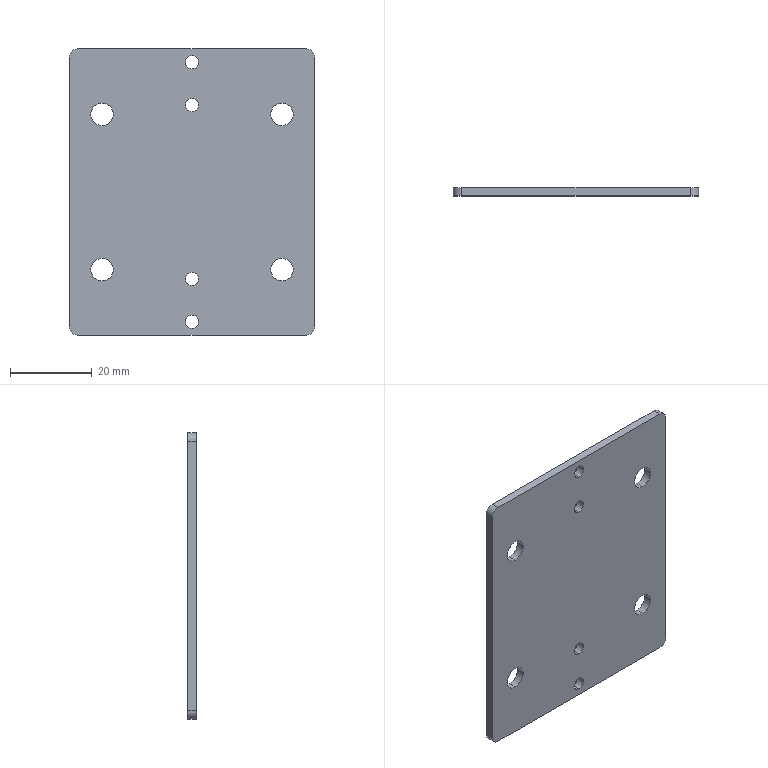Part | SolidWorks | features BaseBody 1 | 1 solid | 26 faces | box 60 x 2 x 70 mm | volume 8139 mm3 | cylinder 20 | plane 6 | commonest cylinder face diameters 3.2 x8 5.5 x8 4 x4
STEP:
#1=CARTESIAN_POINT('',(22.,1.,-16.25));
#2=VERTEX_POINT('',#1);
#3=CARTESIAN_POINT('',(22.,1.,-21.75));
#4=VERTEX_POINT('',#3);
#5=CARTESIAN_POINT('',(22.,1.,-19.));
#6=DIRECTION('',(0.,-1.,0.));
#7=DIRECTION('',(0.,0.,-1.));
#8=AXIS2_PLACEMENT_3D('',#5,#6,#7);
#9=CIRCLE('',#8,2.75);
#10=EDGE_CURVE('',#2,#4,#9,.T.);
#11=ORIENTED_EDGE('',*,*,#10,.F.);
#12=CARTESIAN_POINT('',(22.,-1.,-16.25));
#13=VERTEX_POINT('',#12);
#14=CARTESIAN_POINT('',(22.,1.,-16.25));
#15=DIRECTION('',(0.,-1.,0.));
#16=VECTOR('',#15,1000.);
#17=LINE('',#14,#16);
#18=EDGE_CURVE('',#2,#13,#17,.T.);
#19=ORIENTED_EDGE('',*,*,#18,.T.);
#20=CARTESIAN_POINT('',(22.,-1.,-21.75));
#21=VERTEX_POINT('',#20);
#22=CARTESIAN_POINT('',(22.,-1.,-19.));
#23=DIRECTION('',(0.,1.,0.));
#24=DIRECTION('',(0.,0.,-1.));
#25=AXIS2_PLACEMENT_3D('',#22,#23,#24);
#26=CIRCLE('',#25,2.75);
#27=EDGE_CURVE('',#21,#13,#26,.T.);
#28=ORIENTED_EDGE('',*,*,#27,.F.);
#29=CARTESIAN_POINT('',(22.,1.,-21.75));
#30=DIRECTION('',(0.,-1.,0.));
#31=VECTOR('',#30,1000.);
#32=LINE('',#29,#31);
#33=EDGE_CURVE('',#4,#21,#32,.T.);
#34=ORIENTED_EDGE('',*,*,#33,.F.);
#35=EDGE_LOOP('',(#11,#19,#28,#34));
#36=FACE_OUTER_BOUND('',#35,.T.);
#37=CARTESIAN_POINT('',(22.,1.,-19.));
#38=DIRECTION('',(0.,-1.,0.));
#39=DIRECTION('',(0.,0.,-1.));
#40=AXIS2_PLACEMENT_3D('',#37,#38,#39);
#41=CYLINDRICAL_SURFACE('',#40,2.75);
#42=ADVANCED_FACE('',(#36),#41,.F.);
#43=CARTESIAN_POINT('',(0.,1.,33.35));
#44=VERTEX_POINT('',#43);
#45=CARTESIAN_POINT('',(0.,1.,30.15));
#46=VERTEX_POINT('',#45);
#47=CARTESIAN_POINT('',(0.,1.,31.75));
#48=DIRECTION('',(0.,-1.,0.));
#49=DIRECTION('',(0.,0.,-1.));
#50=AXIS2_PLACEMENT_3D('',#47,#48,#49);
#51=CIRCLE('',#50,1.6);
#52=EDGE_CURVE('',#44,#46,#51,.T.);
#53=ORIENTED_EDGE('',*,*,#52,.F.);
#54=CARTESIAN_POINT('',(0.,-1.,33.35));
#55=VERTEX_POINT('',#54);
#56=CARTESIAN_POINT('',(0.,1.,33.35));
#57=DIRECTION('',(0.,-1.,0.));
#58=VECTOR('',#57,1000.);
#59=LINE('',#56,#58);
#60=EDGE_CURVE('',#44,#55,#59,.T.);
#61=ORIENTED_EDGE('',*,*,#60,.T.);
#62=CARTESIAN_POINT('',(0.,-1.,30.15));
#63=VERTEX_POINT('',#62);
#64=CARTESIAN_POINT('',(0.,-1.,31.75));
#65=DIRECTION('',(0.,1.,0.));
#66=DIRECTION('',(0.,0.,-1.));
#67=AXIS2_PLACEMENT_3D('',#64,#65,#66);
#68=CIRCLE('',#67,1.6);
#69=EDGE_CURVE('',#63,#55,#68,.T.);
#70=ORIENTED_EDGE('',*,*,#69,.F.);
#71=CARTESIAN_POINT('',(0.,1.,30.15));
#72=DIRECTION('',(0.,-1.,0.));
#73=VECTOR('',#72,1000.);
#74=LINE('',#71,#73);
#75=EDGE_CURVE('',#46,#63,#74,.T.);
#76=ORIENTED_EDGE('',*,*,#75,.F.);
#77=EDGE_LOOP('',(#53,#61,#70,#76));
#78=FACE_OUTER_BOUND('',#77,.T.);
#79=CARTESIAN_POINT('',(0.,1.,31.75));
#80=DIRECTION('',(0.,-1.,0.));
#81=DIRECTION('',(0.,0.,-1.));
#82=AXIS2_PLACEMENT_3D('',#79,#80,#81);
#83=CYLINDRICAL_SURFACE('',#82,1.6);
#84=ADVANCED_FACE('',(#78),#83,.F.);
#85=CARTESIAN_POINT('',(0.,1.,-19.65));
#86=VERTEX_POINT('',#85);
#87=CARTESIAN_POINT('',(0.,1.,-22.85));
#88=VERTEX_POINT('',#87);
#89=CARTESIAN_POINT('',(0.,1.,-21.25));
#90=DIRECTION('',(0.,-1.,0.));
#91=DIRECTION('',(0.,0.,-1.));
#92=AXIS2_PLACEMENT_3D('',#89,#90,#91);
#93=CIRCLE('',#92,1.6);
#94=EDGE_CURVE('',#86,#88,#93,.T.);
#95=ORIENTED_EDGE('',*,*,#94,.F.);
#96=CARTESIAN_POINT('',(0.,-1.,-19.65));
#97=VERTEX_POINT('',#96);
#98=CARTESIAN_POINT('',(0.,1.,-19.65));
#99=DIRECTION('',(0.,-1.,0.));
#100=VECTOR('',#99,1000.);
#101=LINE('',#98,#100);
#102=EDGE_CURVE('',#86,#97,#101,.T.);
#103=ORIENTED_EDGE('',*,*,#102,.T.);
#104=CARTESIAN_POINT('',(0.,-1.,-22.85));
#105=VERTEX_POINT('',#104);
#106=CARTESIAN_POINT('',(0.,-1.,-21.25));
#107=DIRECTION('',(0.,1.,0.));
#108=DIRECTION('',(0.,0.,-1.));
#109=AXIS2_PLACEMENT_3D('',#106,#107,#108);
#110=CIRCLE('',#109,1.6);
#111=EDGE_CURVE('',#105,#97,#110,.T.);
#112=ORIENTED_EDGE('',*,*,#111,.F.);
#113=CARTESIAN_POINT('',(0.,1.,-22.85));
#114=DIRECTION('',(0.,-1.,0.));
#115=VECTOR('',#114,1000.);
#116=LINE('',#113,#115);
#117=EDGE_CURVE('',#88,#105,#116,.T.);
#118=ORIENTED_EDGE('',*,*,#117,.F.);
#119=EDGE_LOOP('',(#95,#103,#112,#118));
#120=FACE_OUTER_BOUND('',#119,.T.);
#121=CARTESIAN_POINT('',(0.,1.,-21.25));
#122=DIRECTION('',(0.,-1.,0.));
#123=DIRECTION('',(0.,0.,-1.));
#124=AXIS2_PLACEMENT_3D('',#121,#122,#123);
#125=CYLINDRICAL_SURFACE('',#124,1.6);
#126=ADVANCED_FACE('',(#120),#125,.F.);
#127=CARTESIAN_POINT('',(-22.,1.,21.75));
#128=VERTEX_POINT('',#127);
#129=CARTESIAN_POINT('',(-22.,1.,16.25));
#130=VERTEX_POINT('',#129);
#131=CARTESIAN_POINT('',(-22.,1.,19.));
#132=DIRECTION('',(0.,-1.,0.));
#133=DIRECTION('',(0.,0.,-1.));
#134=AXIS2_PLACEMENT_3D('',#131,#132,#133);
#135=CIRCLE('',#134,2.75);
#136=EDGE_CURVE('',#128,#130,#135,.T.);
#137=ORIENTED_EDGE('',*,*,#136,.F.);
#138=CARTESIAN_POINT('',(-22.,-1.,21.75));
#139=VERTEX_POINT('',#138);
#140=CARTESIAN_POINT('',(-22.,1.,21.75));
#141=DIRECTION('',(0.,-1.,0.));
#142=VECTOR('',#141,1000.);
#143=LINE('',#140,#142);
#144=EDGE_CURVE('',#128,#139,#143,.T.);
#145=ORIENTED_EDGE('',*,*,#144,.T.);
#146=CARTESIAN_POINT('',(-22.,-1.,16.25));
#147=VERTEX_POINT('',#146);
#148=CARTESIAN_POINT('',(-22.,-1.,19.));
#149=DIRECTION('',(0.,1.,0.));
#150=DIRECTION('',(0.,0.,-1.));
#151=AXIS2_PLACEMENT_3D('',#148,#149,#150);
#152=CIRCLE('',#151,2.75);
#153=EDGE_CURVE('',#147,#139,#152,.T.);
#154=ORIENTED_EDGE('',*,*,#153,.F.);
#155=CARTESIAN_POINT('',(-22.,1.,16.25));
#156=DIRECTION('',(0.,-1.,0.));
#157=VECTOR('',#156,1000.);
#158=LINE('',#155,#157);
#159=EDGE_CURVE('',#130,#147,#158,.T.);
#160=ORIENTED_EDGE('',*,*,#159,.F.);
#161=EDGE_LOOP('',(#137,#145,#154,#160));
#162=FACE_OUTER_BOUND('',#161,.T.);
#163=CARTESIAN_POINT('',(-22.,1.,19.));
#164=DIRECTION('',(0.,-1.,0.));
#165=DIRECTION('',(0.,0.,-1.));
#166=AXIS2_PLACEMENT_3D('',#163,#164,#165);
#167=CYLINDRICAL_SURFACE('',#166,2.75);
#168=ADVANCED_FACE('',(#162),#167,.F.);
#169=CARTESIAN_POINT('',(-22.,1.,-16.25));
#170=VERTEX_POINT('',#169);
#171=CARTESIAN_POINT('',(-22.,1.,-21.75));
#172=VERTEX_POINT('',#171);
#173=CARTESIAN_POINT('',(-22.,1.,-19.));
#174=DIRECTION('',(0.,-1.,0.));
#175=DIRECTION('',(0.,0.,-1.));
#176=AXIS2_PLACEMENT_3D('',#173,#174,#175);
#177=CIRCLE('',#176,2.75);
#178=EDGE_CURVE('',#170,#172,#177,.T.);
#179=ORIENTED_EDGE('',*,*,#178,.F.);
#180=CARTESIAN_POINT('',(-22.,-1.,-16.25));
#181=VERTEX_POINT('',#180);
#182=CARTESIAN_POINT('',(-22.,1.,-16.25));
#183=DIRECTION('',(0.,-1.,0.));
#184=VECTOR('',#183,1000.);
#185=LINE('',#182,#184);
#186=EDGE_CURVE('',#170,#181,#185,.T.);
#187=ORIENTED_EDGE('',*,*,#186,.T.);
#188=CARTESIAN_POINT('',(-22.,-1.,-21.75));
#189=VERTEX_POINT('',#188);
#190=CARTESIAN_POINT('',(-22.,-1.,-19.));
#191=DIRECTION('',(0.,1.,0.));
#192=DIRECTION('',(0.,0.,-1.));
#193=AXIS2_PLACEMENT_3D('',#190,#191,#192);
#194=CIRCLE('',#193,2.75);
#195=EDGE_CURVE('',#189,#181,#194,.T.);
#196=ORIENTED_EDGE('',*,*,#195,.F.);
#197=CARTESIAN_POINT('',(-22.,1.,-21.75));
#198=DIRECTION('',(0.,-1.,0.));
#199=VECTOR('',#198,1000.);
#200=LINE('',#197,#199);
#201=EDGE_CURVE('',#172,#189,#200,.T.);
#202=ORIENTED_EDGE('',*,*,#201,.F.);
#203=EDGE_LOOP('',(#179,#187,#196,#202));
#204=FACE_OUTER_BOUND('',#203,.T.);
#205=CARTESIAN_POINT('',(-22.,1.,-19.));
#206=DIRECTION('',(0.,-1.,0.));
#207=DIRECTION('',(0.,0.,-1.));
#208=AXIS2_PLACEMENT_3D('',#205,#206,#207);
#209=CYLINDRICAL_SURFACE('',#208,2.75);
#210=ADVANCED_FACE('',(#204),#209,.F.);
#211=CARTESIAN_POINT('',(0.,1.,-30.15));
#212=VERTEX_POINT('',#211);
#213=CARTESIAN_POINT('',(0.,1.,-33.35));
#214=VERTEX_POINT('',#213);
#215=CARTESIAN_POINT('',(0.,1.,-31.75));
#216=DIRECTION('',(0.,-1.,0.));
#217=DIRECTION('',(0.,0.,-1.));
#218=AXIS2_PLACEMENT_3D('',#215,#216,#217);
#219=CIRCLE('',#218,1.6);
#220=EDGE_CURVE('',#212,#214,#219,.T.);
#221=ORIENTED_EDGE('',*,*,#220,.F.);
#222=CARTESIAN_POINT('',(0.,-1.,-30.15));
#223=VERTEX_POINT('',#222);
#224=CARTESIAN_POINT('',(0.,1.,-30.15));
#225=DIRECTION('',(0.,-1.,0.));
#226=VECTOR('',#225,1000.);
#227=LINE('',#224,#226);
#228=EDGE_CURVE('',#212,#223,#227,.T.);
#229=ORIENTED_EDGE('',*,*,#228,.T.);
#230=CARTESIAN_POINT('',(0.,-1.,-33.35));
#231=VERTEX_POINT('',#230);
#232=CARTESIAN_POINT('',(0.,-1.,-31.75));
#233=DIRECTION('',(0.,1.,0.));
#234=DIRECTION('',(0.,0.,-1.));
#235=AXIS2_PLACEMENT_3D('',#232,#233,#234);
#236=CIRCLE('',#235,1.6);
#237=EDGE_CURVE('',#231,#223,#236,.T.);
#238=ORIENTED_EDGE('',*,*,#237,.F.);
#239=CARTESIAN_POINT('',(0.,1.,-33.35));
#240=DIRECTION('',(0.,-1.,0.));
#241=VECTOR('',#240,1000.);
#242=LINE('',#239,#241);
#243=EDGE_CURVE('',#214,#231,#242,.T.);
#244=ORIENTED_EDGE('',*,*,#243,.F.);
#245=EDGE_LOOP('',(#221,#229,#238,#244));
#246=FACE_OUTER_BOUND('',#245,.T.);
#247=CARTESIAN_POINT('',(0.,1.,-31.75));
#248=DIRECTION('',(0.,-1.,0.));
#249=DIRECTION('',(0.,0.,-1.));
#250=AXIS2_PLACEMENT_3D('',#247,#248,#249);
#251=CYLINDRICAL_SURFACE('',#250,1.6);
#252=ADVANCED_FACE('',(#246),#251,.F.);
#253=CARTESIAN_POINT('',(0.,1.,22.85));
#254=VERTEX_POINT('',#253);
#255=CARTESIAN_POINT('',(0.,1.,19.65));
#256=VERTEX_POINT('',#255);
#257=CARTESIAN_POINT('',(0.,1.,21.25));
#258=DIRECTION('',(0.,-1.,0.));
#259=DIRECTION('',(0.,0.,-1.));
#260=AXIS2_PLACEMENT_3D('',#257,#258,#259);
#261=CIRCLE('',#260,1.6);
#262=EDGE_CURVE('',#254,#256,#261,.T.);
#263=ORIENTED_EDGE('',*,*,#262,.F.);
#264=CARTESIAN_POINT('',(0.,-1.,22.85));
#265=VERTEX_POINT('',#264);
#266=CARTESIAN_POINT('',(0.,1.,22.85));
#267=DIRECTION('',(0.,-1.,0.));
#268=VECTOR('',#267,1000.);
#269=LINE('',#266,#268);
#270=EDGE_CURVE('',#254,#265,#269,.T.);
#271=ORIENTED_EDGE('',*,*,#270,.T.);
#272=CARTESIAN_POINT('',(0.,-1.,19.65));
#273=VERTEX_POINT('',#272);
#274=CARTESIAN_POINT('',(0.,-1.,21.25));
#275=DIRECTION('',(0.,1.,0.));
#276=DIRECTION('',(0.,0.,-1.));
#277=AXIS2_PLACEMENT_3D('',#274,#275,#276);
#278=CIRCLE('',#277,1.6);
#279=EDGE_CURVE('',#273,#265,#278,.T.);
#280=ORIENTED_EDGE('',*,*,#279,.F.);
#281=CARTESIAN_POINT('',(0.,1.,19.65));
#282=DIRECTION('',(0.,-1.,0.));
#283=VECTOR('',#282,1000.);
#284=LINE('',#281,#283);
#285=EDGE_CURVE('',#256,#273,#284,.T.);
#286=ORIENTED_EDGE('',*,*,#285,.F.);
#287=EDGE_LOOP('',(#263,#271,#280,#286));
#288=FACE_OUTER_BOUND('',#287,.T.);
#289=CARTESIAN_POINT('',(0.,1.,21.25));
#290=DIRECTION('',(0.,-1.,0.));
#291=DIRECTION('',(0.,0.,-1.));
#292=AXIS2_PLACEMENT_3D('',#289,#290,#291);
#293=CYLINDRICAL_SURFACE('',#292,1.6);
#294=ADVANCED_FACE('',(#288),#293,.F.);
#295=CARTESIAN_POINT('',(22.,1.,21.75));
#296=VERTEX_POINT('',#295);
#297=CARTESIAN_POINT('',(22.,1.,16.25));
#298=VERTEX_POINT('',#297);
#299=CARTESIAN_POINT('',(22.,1.,19.));
#300=DIRECTION('',(0.,-1.,0.));
#301=DIRECTION('',(0.,0.,-1.));
#302=AXIS2_PLACEMENT_3D('',#299,#300,#301);
#303=CIRCLE('',#302,2.75);
#304=EDGE_CURVE('',#296,#298,#303,.T.);
#305=ORIENTED_EDGE('',*,*,#304,.F.);
#306=CARTESIAN_POINT('',(22.,-1.,21.75));
#307=VERTEX_POINT('',#306);
#308=CARTESIAN_POINT('',(22.,1.,21.75));
#309=DIRECTION('',(0.,-1.,0.));
#310=VECTOR('',#309,1000.);
#311=LINE('',#308,#310);
#312=EDGE_CURVE('',#296,#307,#311,.T.);
#313=ORIENTED_EDGE('',*,*,#312,.T.);
#314=CARTESIAN_POINT('',(22.,-1.,16.25));
#315=VERTEX_POINT('',#314);
#316=CARTESIAN_POINT('',(22.,-1.,19.));
#317=DIRECTION('',(0.,1.,0.));
#318=DIRECTION('',(0.,0.,-1.));
#319=AXIS2_PLACEMENT_3D('',#316,#317,#318);
#320=CIRCLE('',#319,2.75);
#321=EDGE_CURVE('',#315,#307,#320,.T.);
#322=ORIENTED_EDGE('',*,*,#321,.F.);
#323=CARTESIAN_POINT('',(22.,1.,16.25));
#324=DIRECTION('',(0.,-1.,0.));
#325=VECTOR('',#324,1000.);
#326=LINE('',#323,#325);
#327=EDGE_CURVE('',#298,#315,#326,.T.);
#328=ORIENTED_EDGE('',*,*,#327,.F.);
#329=EDGE_LOOP('',(#305,#313,#322,#328));
#330=FACE_OUTER_BOUND('',#329,.T.);
#331=CARTESIAN_POINT('',(22.,1.,19.));
#332=DIRECTION('',(0.,-1.,0.));
#333=DIRECTION('',(0.,0.,-1.));
#334=AXIS2_PLACEMENT_3D('',#331,#332,#333);
#335=CYLINDRICAL_SURFACE('',#334,2.75);
#336=ADVANCED_FACE('',(#330),#335,.F.);
#337=CARTESIAN_POINT('',(22.,1.,-19.));
#338=DIRECTION('',(0.,-1.,0.));
#339=DIRECTION('',(0.,0.,-1.));
#340=AXIS2_PLACEMENT_3D('',#337,#338,#339);
#341=CIRCLE('',#340,2.75);
#342=EDGE_CURVE('',#4,#2,#341,.T.);
#343=ORIENTED_EDGE('',*,*,#342,.T.);
#344=ORIENTED_EDGE('',*,*,#10,.T.);
#345=EDGE_LOOP('',(#343,#344));
#346=FACE_BOUND('',#345,.T.);
#347=CARTESIAN_POINT('',(0.,1.,31.75));
#348=DIRECTION('',(0.,-1.,0.));
#349=DIRECTION('',(0.,0.,-1.));
#350=AXIS2_PLACEMENT_3D('',#347,#348,#349);
#351=CIRCLE('',#350,1.6);
#352=EDGE_CURVE('',#46,#44,#351,.T.);
#353=ORIENTED_EDGE('',*,*,#352,.T.);
#354=ORIENTED_EDGE('',*,*,#52,.T.);
#355=EDGE_LOOP('',(#353,#354));
#356=FACE_BOUND('',#355,.T.);
#357=CARTESIAN_POINT('',(0.,1.,-21.25));
#358=DIRECTION('',(0.,-1.,0.));
#359=DIRECTION('',(0.,0.,-1.));
#360=AXIS2_PLACEMENT_3D('',#357,#358,#359);
#361=CIRCLE('',#360,1.6);
#362=EDGE_CURVE('',#88,#86,#361,.T.);
#363=ORIENTED_EDGE('',*,*,#362,.T.);
#364=ORIENTED_EDGE('',*,*,#94,.T.);
#365=EDGE_LOOP('',(#363,#364));
#366=FACE_BOUND('',#365,.T.);
#367=CARTESIAN_POINT('',(-22.,1.,19.));
#368=DIRECTION('',(0.,-1.,0.));
#369=DIRECTION('',(0.,0.,-1.));
#370=AXIS2_PLACEMENT_3D('',#367,#368,#369);
#371=CIRCLE('',#370,2.75);
#372=EDGE_CURVE('',#130,#128,#371,.T.);
#373=ORIENTED_EDGE('',*,*,#372,.T.);
#374=ORIENTED_EDGE('',*,*,#136,.T.);
#375=EDGE_LOOP('',(#373,#374));
#376=FACE_BOUND('',#375,.T.);
#377=CARTESIAN_POINT('',(-30.,1.,-33.));
#378=VERTEX_POINT('',#377);
#379=CARTESIAN_POINT('',(-30.,1.,33.));
#380=VERTEX_POINT('',#379);
#381=CARTESIAN_POINT('',(-30.,1.,0.));
#382=DIRECTION('',(0.,0.,1.));
#383=VECTOR('',#382,1000.);
#384=LINE('',#381,#383);
#385=EDGE_CURVE('',#378,#380,#384,.T.);
#386=ORIENTED_EDGE('',*,*,#385,.T.);
#387=CARTESIAN_POINT('',(-28.,1.,35.));
#388=VERTEX_POINT('',#387);
#389=CARTESIAN_POINT('',(-28.,1.,33.));
#390=DIRECTION('',(0.,1.,0.));
#391=DIRECTION('',(0.,0.,-1.));
#392=AXIS2_PLACEMENT_3D('',#389,#390,#391);
#393=CIRCLE('',#392,2.);
#394=EDGE_CURVE('',#380,#388,#393,.T.);
#395=ORIENTED_EDGE('',*,*,#394,.T.);
#396=CARTESIAN_POINT('',(28.,1.,35.));
#397=VERTEX_POINT('',#396);
#398=CARTESIAN_POINT('',(0.,1.,35.));
#399=DIRECTION('',(1.,0.,0.));
#400=VECTOR('',#399,1000.);
#401=LINE('',#398,#400);
#402=EDGE_CURVE('',#388,#397,#401,.T.);
#403=ORIENTED_EDGE('',*,*,#402,.T.);
#404=CARTESIAN_POINT('',(30.,1.,33.));
#405=VERTEX_POINT('',#404);
#406=CARTESIAN_POINT('',(28.,1.,33.));
#407=DIRECTION('',(0.,1.,0.));
#408=DIRECTION('',(0.,0.,-1.));
#409=AXIS2_PLACEMENT_3D('',#406,#407,#408);
#410=CIRCLE('',#409,2.);
#411=EDGE_CURVE('',#397,#405,#410,.T.);
#412=ORIENTED_EDGE('',*,*,#411,.T.);
#413=CARTESIAN_POINT('',(30.,1.,-33.));
#414=VERTEX_POINT('',#413);
#415=CARTESIAN_POINT('',(30.,1.,0.));
#416=DIRECTION('',(0.,0.,-1.));
#417=VECTOR('',#416,1000.);
#418=LINE('',#415,#417);
#419=EDGE_CURVE('',#405,#414,#418,.T.);
#420=ORIENTED_EDGE('',*,*,#419,.T.);
#421=CARTESIAN_POINT('',(28.,1.,-35.));
#422=VERTEX_POINT('',#421);
#423=CARTESIAN_POINT('',(28.,1.,-33.));
#424=DIRECTION('',(0.,1.,0.));
#425=DIRECTION('',(0.,0.,-1.));
#426=AXIS2_PLACEMENT_3D('',#423,#424,#425);
#427=CIRCLE('',#426,2.);
#428=EDGE_CURVE('',#414,#422,#427,.T.);
#429=ORIENTED_EDGE('',*,*,#428,.T.);
#430=CARTESIAN_POINT('',(-28.,1.,-35.));
#431=VERTEX_POINT('',#430);
#432=CARTESIAN_POINT('',(0.,1.,-35.));
#433=DIRECTION('',(-1.,0.,0.));
#434=VECTOR('',#433,1000.);
#435=LINE('',#432,#434);
#436=EDGE_CURVE('',#422,#431,#435,.T.);
#437=ORIENTED_EDGE('',*,*,#436,.T.);
#438=CARTESIAN_POINT('',(-28.,1.,-33.));
#439=DIRECTION('',(0.,1.,0.));
#440=DIRECTION('',(0.,0.,-1.));
#441=AXIS2_PLACEMENT_3D('',#438,#439,#440);
#442=CIRCLE('',#441,2.);
#443=EDGE_CURVE('',#431,#378,#442,.T.);
#444=ORIENTED_EDGE('',*,*,#443,.T.);
#445=EDGE_LOOP('',(#386,#395,#403,#412,#420,#429,#437,#444));
#446=FACE_OUTER_BOUND('',#445,.T.);
#447=CARTESIAN_POINT('',(-22.,1.,-19.));
#448=DIRECTION('',(0.,-1.,0.));
#449=DIRECTION('',(0.,0.,-1.));
#450=AXIS2_PLACEMENT_3D('',#447,#448,#449);
#451=CIRCLE('',#450,2.75);
#452=EDGE_CURVE('',#172,#170,#451,.T.);
#453=ORIENTED_EDGE('',*,*,#452,.T.);
#454=ORIENTED_EDGE('',*,*,#178,.T.);
#455=EDGE_LOOP('',(#453,#454));
#456=FACE_BOUND('',#455,.T.);
#457=CARTESIAN_POINT('',(0.,1.,-31.75));
#458=DIRECTION('',(0.,-1.,0.));
#459=DIRECTION('',(0.,0.,-1.));
#460=AXIS2_PLACEMENT_3D('',#457,#458,#459);
#461=CIRCLE('',#460,1.6);
#462=EDGE_CURVE('',#214,#212,#461,.T.);
#463=ORIENTED_EDGE('',*,*,#462,.T.);
#464=ORIENTED_EDGE('',*,*,#220,.T.);
#465=EDGE_LOOP('',(#463,#464));
#466=FACE_BOUND('',#465,.T.);
#467=CARTESIAN_POINT('',(0.,1.,21.25));
#468=DIRECTION('',(0.,-1.,0.));
#469=DIRECTION('',(0.,0.,-1.));
#470=AXIS2_PLACEMENT_3D('',#467,#468,#469);
#471=CIRCLE('',#470,1.6);
#472=EDGE_CURVE('',#256,#254,#471,.T.);
#473=ORIENTED_EDGE('',*,*,#472,.T.);
#474=ORIENTED_EDGE('',*,*,#262,.T.);
#475=EDGE_LOOP('',(#473,#474));
#476=FACE_BOUND('',#475,.T.);
#477=CARTESIAN_POINT('',(22.,1.,19.));
#478=DIRECTION('',(0.,-1.,0.));
#479=DIRECTION('',(0.,0.,-1.));
#480=AXIS2_PLACEMENT_3D('',#477,#478,#479);
#481=CIRCLE('',#480,2.75);
#482=EDGE_CURVE('',#298,#296,#481,.T.);
#483=ORIENTED_EDGE('',*,*,#482,.T.);
#484=ORIENTED_EDGE('',*,*,#304,.T.);
#485=EDGE_LOOP('',(#483,#484));
#486=FACE_BOUND('',#485,.T.);
#487=CARTESIAN_POINT('',(0.,1.,0.));
#488=DIRECTION('',(0.,1.,0.));
#489=DIRECTION('',(0.,0.,1.));
#490=AXIS2_PLACEMENT_3D('',#487,#488,#489);
#491=PLANE('',#490);
#492=ADVANCED_FACE('',(#346,#356,#366,#376,#446,#456,#466,#476,#486),#491,.T.);
#493=ORIENTED_EDGE('',*,*,#18,.F.);
#494=ORIENTED_EDGE('',*,*,#342,.F.);
#495=ORIENTED_EDGE('',*,*,#33,.T.);
#496=CARTESIAN_POINT('',(22.,-1.,-19.));
#497=DIRECTION('',(0.,1.,0.));
#498=DIRECTION('',(0.,0.,-1.));
#499=AXIS2_PLACEMENT_3D('',#496,#497,#498);
#500=CIRCLE('',#499,2.75);
#501=EDGE_CURVE('',#13,#21,#500,.T.);
#502=ORIENTED_EDGE('',*,*,#501,.F.);
#503=EDGE_LOOP('',(#493,#494,#495,#502));
#504=FACE_OUTER_BOUND('',#503,.T.);
#505=CARTESIAN_POINT('',(22.,1.,-19.));
#506=DIRECTION('',(0.,-1.,0.));
#507=DIRECTION('',(0.,0.,-1.));
#508=AXIS2_PLACEMENT_3D('',#505,#506,#507);
#509=CYLINDRICAL_SURFACE('',#508,2.75);
#510=ADVANCED_FACE('',(#504),#509,.F.);
#511=ORIENTED_EDGE('',*,*,#60,.F.);
#512=ORIENTED_EDGE('',*,*,#352,.F.);
#513=ORIENTED_EDGE('',*,*,#75,.T.);
#514=CARTESIAN_POINT('',(0.,-1.,31.75));
#515=DIRECTION('',(0.,1.,0.));
#516=DIRECTION('',(0.,0.,-1.));
#517=AXIS2_PLACEMENT_3D('',#514,#515,#516);
#518=CIRCLE('',#517,1.6);
#519=EDGE_CURVE('',#55,#63,#518,.T.);
#520=ORIENTED_EDGE('',*,*,#519,.F.);
#521=EDGE_LOOP('',(#511,#512,#513,#520));
#522=FACE_OUTER_BOUND('',#521,.T.);
#523=CARTESIAN_POINT('',(0.,1.,31.75));
#524=DIRECTION('',(0.,-1.,0.));
#525=DIRECTION('',(0.,0.,-1.));
#526=AXIS2_PLACEMENT_3D('',#523,#524,#525);
#527=CYLINDRICAL_SURFACE('',#526,1.6);
#528=ADVANCED_FACE('',(#522),#527,.F.);
#529=ORIENTED_EDGE('',*,*,#102,.F.);
#530=ORIENTED_EDGE('',*,*,#362,.F.);
#531=ORIENTED_EDGE('',*,*,#117,.T.);
#532=CARTESIAN_POINT('',(0.,-1.,-21.25));
#533=DIRECTION('',(0.,1.,0.));
#534=DIRECTION('',(0.,0.,-1.));
#535=AXIS2_PLACEMENT_3D('',#532,#533,#534);
#536=CIRCLE('',#535,1.6);
#537=EDGE_CURVE('',#97,#105,#536,.T.);
#538=ORIENTED_EDGE('',*,*,#537,.F.);
#539=EDGE_LOOP('',(#529,#530,#531,#538));
#540=FACE_OUTER_BOUND('',#539,.T.);
#541=CARTESIAN_POINT('',(0.,1.,-21.25));
#542=DIRECTION('',(0.,-1.,0.));
#543=DIRECTION('',(0.,0.,-1.));
#544=AXIS2_PLACEMENT_3D('',#541,#542,#543);
#545=CYLINDRICAL_SURFACE('',#544,1.6);
#546=ADVANCED_FACE('',(#540),#545,.F.);
#547=ORIENTED_EDGE('',*,*,#144,.F.);
#548=ORIENTED_EDGE('',*,*,#372,.F.);
#549=ORIENTED_EDGE('',*,*,#159,.T.);
#550=CARTESIAN_POINT('',(-22.,-1.,19.));
#551=DIRECTION('',(0.,1.,0.));
#552=DIRECTION('',(0.,0.,-1.));
#553=AXIS2_PLACEMENT_3D('',#550,#551,#552);
#554=CIRCLE('',#553,2.75);
#555=EDGE_CURVE('',#139,#147,#554,.T.);
#556=ORIENTED_EDGE('',*,*,#555,.F.);
#557=EDGE_LOOP('',(#547,#548,#549,#556));
#558=FACE_OUTER_BOUND('',#557,.T.);
#559=CARTESIAN_POINT('',(-22.,1.,19.));
#560=DIRECTION('',(0.,-1.,0.));
#561=DIRECTION('',(0.,0.,-1.));
#562=AXIS2_PLACEMENT_3D('',#559,#560,#561);
#563=CYLINDRICAL_SURFACE('',#562,2.75);
#564=ADVANCED_FACE('',(#558),#563,.F.);
#565=CARTESIAN_POINT('',(-30.,-1.,33.));
#566=VERTEX_POINT('',#565);
#567=CARTESIAN_POINT('',(-28.,-1.,35.));
#568=VERTEX_POINT('',#567);
#569=CARTESIAN_POINT('',(-28.,-1.,33.));
#570=DIRECTION('',(0.,1.,0.));
#571=DIRECTION('',(0.,0.,-1.));
#572=AXIS2_PLACEMENT_3D('',#569,#570,#571);
#573=CIRCLE('',#572,2.);
#574=EDGE_CURVE('',#566,#568,#573,.T.);
#575=ORIENTED_EDGE('',*,*,#574,.T.);
#576=CARTESIAN_POINT('',(-28.,1.,35.));
#577=DIRECTION('',(0.,1.,0.));
#578=VECTOR('',#577,1000.);
#579=LINE('',#576,#578);
#580=EDGE_CURVE('',#568,#388,#579,.T.);
#581=ORIENTED_EDGE('',*,*,#580,.T.);
#582=ORIENTED_EDGE('',*,*,#394,.F.);
#583=CARTESIAN_POINT('',(-30.,1.,33.));
#584=DIRECTION('',(0.,-1.,0.));
#585=VECTOR('',#584,1000.);
#586=LINE('',#583,#585);
#587=EDGE_CURVE('',#380,#566,#586,.T.);
#588=ORIENTED_EDGE('',*,*,#587,.T.);
#589=EDGE_LOOP('',(#575,#581,#582,#588));
#590=FACE_OUTER_BOUND('',#589,.T.);
#591=CARTESIAN_POINT('',(-28.,1.,33.));
#592=DIRECTION('',(0.,-1.,0.));
#593=DIRECTION('',(0.,0.,-1.));
#594=AXIS2_PLACEMENT_3D('',#591,#592,#593);
#595=CYLINDRICAL_SURFACE('',#594,2.);
#596=ADVANCED_FACE('',(#590),#595,.T.);
#597=ORIENTED_EDGE('',*,*,#587,.F.);
#598=ORIENTED_EDGE('',*,*,#385,.F.);
#599=CARTESIAN_POINT('',(-30.,-1.,-33.));
#600=VERTEX_POINT('',#599);
#601=CARTESIAN_POINT('',(-30.,1.,-33.));
#602=DIRECTION('',(0.,1.,0.));
#603=VECTOR('',#602,1000.);
#604=LINE('',#601,#603);
#605=EDGE_CURVE('',#600,#378,#604,.T.);
#606=ORIENTED_EDGE('',*,*,#605,.F.);
#607=CARTESIAN_POINT('',(-30.,-1.,35.));
#608=DIRECTION('',(0.,0.,-1.));
#609=VECTOR('',#608,1000.);
#610=LINE('',#607,#609);
#611=EDGE_CURVE('',#566,#600,#610,.T.);
#612=ORIENTED_EDGE('',*,*,#611,.F.);
#613=EDGE_LOOP('',(#597,#598,#606,#612));
#614=FACE_OUTER_BOUND('',#613,.T.);
#615=CARTESIAN_POINT('',(-30.,1.,35.));
#616=DIRECTION('',(1.,0.,0.));
#617=DIRECTION('',(0.,0.,-1.));
#618=AXIS2_PLACEMENT_3D('',#615,#616,#617);
#619=PLANE('',#618);
#620=ADVANCED_FACE('',(#614),#619,.F.);
#621=CARTESIAN_POINT('',(-28.,-1.,-35.));
#622=VERTEX_POINT('',#621);
#623=CARTESIAN_POINT('',(-28.,-1.,-33.));
#624=DIRECTION('',(0.,1.,0.));
#625=DIRECTION('',(0.,0.,-1.));
#626=AXIS2_PLACEMENT_3D('',#623,#624,#625);
#627=CIRCLE('',#626,2.);
#628=EDGE_CURVE('',#622,#600,#627,.T.);
#629=ORIENTED_EDGE('',*,*,#628,.T.);
#630=ORIENTED_EDGE('',*,*,#605,.T.);
#631=ORIENTED_EDGE('',*,*,#443,.F.);
#632=CARTESIAN_POINT('',(-28.,1.,-35.));
#633=DIRECTION('',(0.,-1.,0.));
#634=VECTOR('',#633,1000.);
#635=LINE('',#632,#634);
#636=EDGE_CURVE('',#431,#622,#635,.T.);
#637=ORIENTED_EDGE('',*,*,#636,.T.);
#638=EDGE_LOOP('',(#629,#630,#631,#637));
#639=FACE_OUTER_BOUND('',#638,.T.);
#640=CARTESIAN_POINT('',(-28.,1.,-33.));
#641=DIRECTION('',(0.,-1.,0.));
#642=DIRECTION('',(0.,0.,-1.));
#643=AXIS2_PLACEMENT_3D('',#640,#641,#642);
#644=CYLINDRICAL_SURFACE('',#643,2.);
#645=ADVANCED_FACE('',(#639),#644,.T.);
#646=CARTESIAN_POINT('',(28.,-1.,-35.));
#647=VERTEX_POINT('',#646);
#648=CARTESIAN_POINT('',(28.,1.,-35.));
#649=DIRECTION('',(0.,1.,0.));
#650=VECTOR('',#649,1000.);
#651=LINE('',#648,#650);
#652=EDGE_CURVE('',#647,#422,#651,.T.);
#653=ORIENTED_EDGE('',*,*,#652,.F.);
#654=CARTESIAN_POINT('',(30.,-1.,-35.));
#655=DIRECTION('',(1.,0.,0.));
#656=VECTOR('',#655,1000.);
#657=LINE('',#654,#656);
#658=EDGE_CURVE('',#622,#647,#657,.T.);
#659=ORIENTED_EDGE('',*,*,#658,.F.);
#660=ORIENTED_EDGE('',*,*,#636,.F.);
#661=ORIENTED_EDGE('',*,*,#436,.F.);
#662=EDGE_LOOP('',(#653,#659,#660,#661));
#663=FACE_OUTER_BOUND('',#662,.T.);
#664=CARTESIAN_POINT('',(30.,1.,-35.));
#665=DIRECTION('',(0.,0.,1.));
#666=DIRECTION('',(1.,0.,0.));
#667=AXIS2_PLACEMENT_3D('',#664,#665,#666);
#668=PLANE('',#667);
#669=ADVANCED_FACE('',(#663),#668,.F.);
#670=CARTESIAN_POINT('',(30.,-1.,-33.));
#671=VERTEX_POINT('',#670);
#672=CARTESIAN_POINT('',(28.,-1.,-33.));
#673=DIRECTION('',(0.,1.,0.));
#674=DIRECTION('',(0.,0.,-1.));
#675=AXIS2_PLACEMENT_3D('',#672,#673,#674);
#676=CIRCLE('',#675,2.);
#677=EDGE_CURVE('',#671,#647,#676,.T.);
#678=ORIENTED_EDGE('',*,*,#677,.T.);
#679=ORIENTED_EDGE('',*,*,#652,.T.);
#680=ORIENTED_EDGE('',*,*,#428,.F.);
#681=CARTESIAN_POINT('',(30.,1.,-33.));
#682=DIRECTION('',(0.,-1.,0.));
#683=VECTOR('',#682,1000.);
#684=LINE('',#681,#683);
#685=EDGE_CURVE('',#414,#671,#684,.T.);
#686=ORIENTED_EDGE('',*,*,#685,.T.);
#687=EDGE_LOOP('',(#678,#679,#680,#686));
#688=FACE_OUTER_BOUND('',#687,.T.);
#689=CARTESIAN_POINT('',(28.,1.,-33.));
#690=DIRECTION('',(0.,-1.,0.));
#691=DIRECTION('',(0.,0.,-1.));
#692=AXIS2_PLACEMENT_3D('',#689,#690,#691);
#693=CYLINDRICAL_SURFACE('',#692,2.);
#694=ADVANCED_FACE('',(#688),#693,.T.);
#695=CARTESIAN_POINT('',(30.,-1.,33.));
#696=VERTEX_POINT('',#695);
#697=CARTESIAN_POINT('',(30.,1.,33.));
#698=DIRECTION('',(0.,1.,0.));
#699=VECTOR('',#698,1000.);
#700=LINE('',#697,#699);
#701=EDGE_CURVE('',#696,#405,#700,.T.);
#702=ORIENTED_EDGE('',*,*,#701,.F.);
#703=CARTESIAN_POINT('',(30.,-1.,35.));
#704=DIRECTION('',(0.,0.,1.));
#705=VECTOR('',#704,1000.);
#706=LINE('',#703,#705);
#707=EDGE_CURVE('',#671,#696,#706,.T.);
#708=ORIENTED_EDGE('',*,*,#707,.F.);
#709=ORIENTED_EDGE('',*,*,#685,.F.);
#710=ORIENTED_EDGE('',*,*,#419,.F.);
#711=EDGE_LOOP('',(#702,#708,#709,#710));
#712=FACE_OUTER_BOUND('',#711,.T.);
#713=CARTESIAN_POINT('',(30.,1.,35.));
#714=DIRECTION('',(-1.,0.,0.));
#715=DIRECTION('',(0.,0.,1.));
#716=AXIS2_PLACEMENT_3D('',#713,#714,#715);
#717=PLANE('',#716);
#718=ADVANCED_FACE('',(#712),#717,.F.);
#719=CARTESIAN_POINT('',(28.,-1.,35.));
#720=VERTEX_POINT('',#719);
#721=CARTESIAN_POINT('',(28.,-1.,33.));
#722=DIRECTION('',(0.,1.,0.));
#723=DIRECTION('',(0.,0.,-1.));
#724=AXIS2_PLACEMENT_3D('',#721,#722,#723);
#725=CIRCLE('',#724,2.);
#726=EDGE_CURVE('',#720,#696,#725,.T.);
#727=ORIENTED_EDGE('',*,*,#726,.T.);
#728=ORIENTED_EDGE('',*,*,#701,.T.);
#729=ORIENTED_EDGE('',*,*,#411,.F.);
#730=CARTESIAN_POINT('',(28.,1.,35.));
#731=DIRECTION('',(0.,-1.,0.));
#732=VECTOR('',#731,1000.);
#733=LINE('',#730,#732);
#734=EDGE_CURVE('',#397,#720,#733,.T.);
#735=ORIENTED_EDGE('',*,*,#734,.T.);
#736=EDGE_LOOP('',(#727,#728,#729,#735));
#737=FACE_OUTER_BOUND('',#736,.T.);
#738=CARTESIAN_POINT('',(28.,1.,33.));
#739=DIRECTION('',(0.,-1.,0.));
#740=DIRECTION('',(0.,0.,-1.));
#741=AXIS2_PLACEMENT_3D('',#738,#739,#740);
#742=CYLINDRICAL_SURFACE('',#741,2.);
#743=ADVANCED_FACE('',(#737),#742,.T.);
#744=ORIENTED_EDGE('',*,*,#734,.F.);
#745=ORIENTED_EDGE('',*,*,#402,.F.);
#746=ORIENTED_EDGE('',*,*,#580,.F.);
#747=CARTESIAN_POINT('',(30.,-1.,35.));
#748=DIRECTION('',(-1.,0.,0.));
#749=VECTOR('',#748,1000.);
#750=LINE('',#747,#749);
#751=EDGE_CURVE('',#720,#568,#750,.T.);
#752=ORIENTED_EDGE('',*,*,#751,.F.);
#753=EDGE_LOOP('',(#744,#745,#746,#752));
#754=FACE_OUTER_BOUND('',#753,.T.);
#755=CARTESIAN_POINT('',(30.,1.,35.));
#756=DIRECTION('',(0.,0.,-1.));
#757=DIRECTION('',(-1.,0.,0.));
#758=AXIS2_PLACEMENT_3D('',#755,#756,#757);
#759=PLANE('',#758);
#760=ADVANCED_FACE('',(#754),#759,.F.);
#761=ORIENTED_EDGE('',*,*,#186,.F.);
#762=ORIENTED_EDGE('',*,*,#452,.F.);
#763=ORIENTED_EDGE('',*,*,#201,.T.);
#764=CARTESIAN_POINT('',(-22.,-1.,-19.));
#765=DIRECTION('',(0.,1.,0.));
#766=DIRECTION('',(0.,0.,-1.));
#767=AXIS2_PLACEMENT_3D('',#764,#765,#766);
#768=CIRCLE('',#767,2.75);
#769=EDGE_CURVE('',#181,#189,#768,.T.);
#770=ORIENTED_EDGE('',*,*,#769,.F.);
#771=EDGE_LOOP('',(#761,#762,#763,#770));
#772=FACE_OUTER_BOUND('',#771,.T.);
#773=CARTESIAN_POINT('',(-22.,1.,-19.));
#774=DIRECTION('',(0.,-1.,0.));
#775=DIRECTION('',(0.,0.,-1.));
#776=AXIS2_PLACEMENT_3D('',#773,#774,#775);
#777=CYLINDRICAL_SURFACE('',#776,2.75);
#778=ADVANCED_FACE('',(#772),#777,.F.);
#779=ORIENTED_EDGE('',*,*,#228,.F.);
#780=ORIENTED_EDGE('',*,*,#462,.F.);
#781=ORIENTED_EDGE('',*,*,#243,.T.);
#782=CARTESIAN_POINT('',(0.,-1.,-31.75));
#783=DIRECTION('',(0.,1.,0.));
#784=DIRECTION('',(0.,0.,-1.));
#785=AXIS2_PLACEMENT_3D('',#782,#783,#784);
#786=CIRCLE('',#785,1.6);
#787=EDGE_CURVE('',#223,#231,#786,.T.);
#788=ORIENTED_EDGE('',*,*,#787,.F.);
#789=EDGE_LOOP('',(#779,#780,#781,#788));
#790=FACE_OUTER_BOUND('',#789,.T.);
#791=CARTESIAN_POINT('',(0.,1.,-31.75));
#792=DIRECTION('',(0.,-1.,0.));
#793=DIRECTION('',(0.,0.,-1.));
#794=AXIS2_PLACEMENT_3D('',#791,#792,#793);
#795=CYLINDRICAL_SURFACE('',#794,1.6);
#796=ADVANCED_FACE('',(#790),#795,.F.);
#797=ORIENTED_EDGE('',*,*,#270,.F.);
#798=ORIENTED_EDGE('',*,*,#472,.F.);
#799=ORIENTED_EDGE('',*,*,#285,.T.);
#800=CARTESIAN_POINT('',(0.,-1.,21.25));
#801=DIRECTION('',(0.,1.,0.));
#802=DIRECTION('',(0.,0.,-1.));
#803=AXIS2_PLACEMENT_3D('',#800,#801,#802);
#804=CIRCLE('',#803,1.6);
#805=EDGE_CURVE('',#265,#273,#804,.T.);
#806=ORIENTED_EDGE('',*,*,#805,.F.);
#807=EDGE_LOOP('',(#797,#798,#799,#806));
#808=FACE_OUTER_BOUND('',#807,.T.);
#809=CARTESIAN_POINT('',(0.,1.,21.25));
#810=DIRECTION('',(0.,-1.,0.));
#811=DIRECTION('',(0.,0.,-1.));
#812=AXIS2_PLACEMENT_3D('',#809,#810,#811);
#813=CYLINDRICAL_SURFACE('',#812,1.6);
#814=ADVANCED_FACE('',(#808),#813,.F.);
#815=ORIENTED_EDGE('',*,*,#312,.F.);
#816=ORIENTED_EDGE('',*,*,#482,.F.);
#817=ORIENTED_EDGE('',*,*,#327,.T.);
#818=CARTESIAN_POINT('',(22.,-1.,19.));
#819=DIRECTION('',(0.,1.,0.));
#820=DIRECTION('',(0.,0.,-1.));
#821=AXIS2_PLACEMENT_3D('',#818,#819,#820);
#822=CIRCLE('',#821,2.75);
#823=EDGE_CURVE('',#307,#315,#822,.T.);
#824=ORIENTED_EDGE('',*,*,#823,.F.);
#825=EDGE_LOOP('',(#815,#816,#817,#824));
#826=FACE_OUTER_BOUND('',#825,.T.);
#827=CARTESIAN_POINT('',(22.,1.,19.));
#828=DIRECTION('',(0.,-1.,0.));
#829=DIRECTION('',(0.,0.,-1.));
#830=AXIS2_PLACEMENT_3D('',#827,#828,#829);
#831=CYLINDRICAL_SURFACE('',#830,2.75);
#832=ADVANCED_FACE('',(#826),#831,.F.);
#833=ORIENTED_EDGE('',*,*,#27,.T.);
#834=ORIENTED_EDGE('',*,*,#501,.T.);
#835=EDGE_LOOP('',(#833,#834));
#836=FACE_BOUND('',#835,.T.);
#837=ORIENTED_EDGE('',*,*,#321,.T.);
#838=ORIENTED_EDGE('',*,*,#823,.T.);
#839=EDGE_LOOP('',(#837,#838));
#840=FACE_BOUND('',#839,.T.);
#841=ORIENTED_EDGE('',*,*,#69,.T.);
#842=ORIENTED_EDGE('',*,*,#519,.T.);
#843=EDGE_LOOP('',(#841,#842));
#844=FACE_BOUND('',#843,.T.);
#845=ORIENTED_EDGE('',*,*,#279,.T.);
#846=ORIENTED_EDGE('',*,*,#805,.T.);
#847=EDGE_LOOP('',(#845,#846));
#848=FACE_BOUND('',#847,.T.);
#849=ORIENTED_EDGE('',*,*,#111,.T.);
#850=ORIENTED_EDGE('',*,*,#537,.T.);
#851=EDGE_LOOP('',(#849,#850));
#852=FACE_BOUND('',#851,.T.);
#853=ORIENTED_EDGE('',*,*,#237,.T.);
#854=ORIENTED_EDGE('',*,*,#787,.T.);
#855=EDGE_LOOP('',(#853,#854));
#856=FACE_BOUND('',#855,.T.);
#857=ORIENTED_EDGE('',*,*,#153,.T.);
#858=ORIENTED_EDGE('',*,*,#555,.T.);
#859=EDGE_LOOP('',(#857,#858));
#860=FACE_BOUND('',#859,.T.);
#861=ORIENTED_EDGE('',*,*,#195,.T.);
#862=ORIENTED_EDGE('',*,*,#769,.T.);
#863=EDGE_LOOP('',(#861,#862));
#864=FACE_BOUND('',#863,.T.);
#865=ORIENTED_EDGE('',*,*,#726,.F.);
#866=ORIENTED_EDGE('',*,*,#751,.T.);
#867=ORIENTED_EDGE('',*,*,#574,.F.);
#868=ORIENTED_EDGE('',*,*,#611,.T.);
#869=ORIENTED_EDGE('',*,*,#628,.F.);
#870=ORIENTED_EDGE('',*,*,#658,.T.);
#871=ORIENTED_EDGE('',*,*,#677,.F.);
#872=ORIENTED_EDGE('',*,*,#707,.T.);
#873=EDGE_LOOP('',(#865,#866,#867,#868,#869,#870,#871,#872));
#874=FACE_OUTER_BOUND('',#873,.T.);
#875=CARTESIAN_POINT('',(0.,-1.,0.));
#876=DIRECTION('',(0.,1.,0.));
#877=DIRECTION('',(0.,0.,1.));
#878=AXIS2_PLACEMENT_3D('',#875,#876,#877);
#879=PLANE('',#878);
#880=ADVANCED_FACE('',(#836,#840,#844,#848,#852,#856,#860,#864,#874),#879,.F.);
#881=CLOSED_SHELL('',(#42,#84,#126,#168,#210,#252,#294,#336,#492,#510,#528,#546,#564,#596,#620,#645,#669,#694,#718,#743,#760,#778,#796,#814,#832,#880));
#882=MANIFOLD_SOLID_BREP('',#881);
#883=CARTESIAN_POINT('',(0.,0.,0.));
#884=DIRECTION('',(0.,0.,1.));
#885=DIRECTION('',(1.,0.,0.));
#886=AXIS2_PLACEMENT_3D('',#883,#884,#885);
#887=(LENGTH_UNIT()NAMED_UNIT(*)SI_UNIT(.MILLI.,.METRE.));
#888=UNCERTAINTY_MEASURE_WITH_UNIT(LENGTH_MEASURE(0.00001),#887,'','');
#889=(NAMED_UNIT(*)PLANE_ANGLE_UNIT()SI_UNIT($,.RADIAN.));
#890=(NAMED_UNIT(*)SI_UNIT($,.STERADIAN.)SOLID_ANGLE_UNIT());
#891=(GEOMETRIC_REPRESENTATION_CONTEXT(3)GLOBAL_UNCERTAINTY_ASSIGNED_CONTEXT((#888))GLOBAL_UNIT_ASSIGNED_CONTEXT((#887,#889,#890))REPRESENTATION_CONTEXT('',''));
#892=ADVANCED_BREP_SHAPE_REPRESENTATION('',(#882,#886),#891);